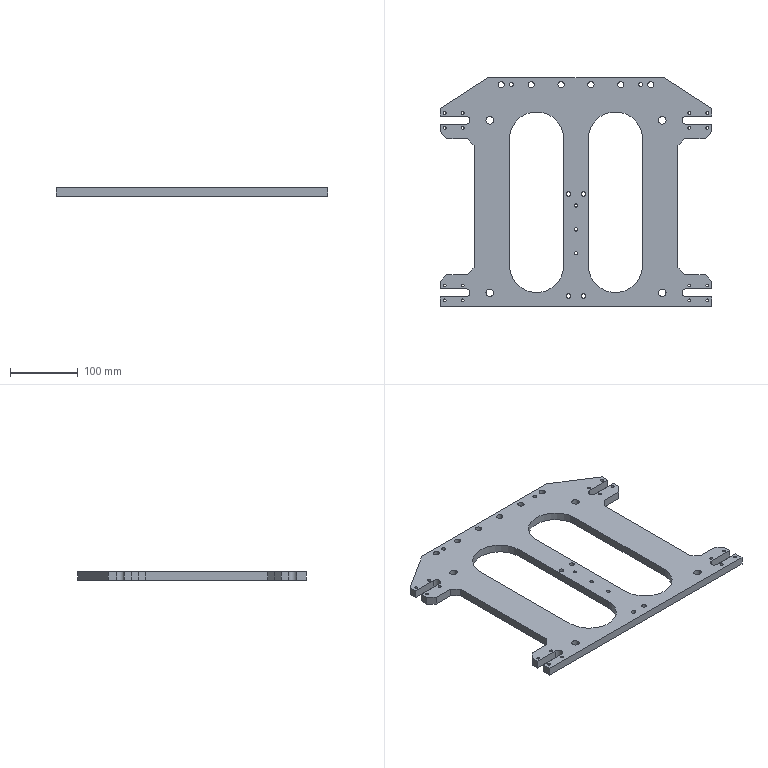Part | 1 solid | 83 faces | box 400 x 336 x 12 mm | volume 817811 mm3 | cylinder 43 | plane 40 | commonest cylinder face diameters 4.2 x16 9 x6 6.6 x4 11 x4 12 x4 80 x4